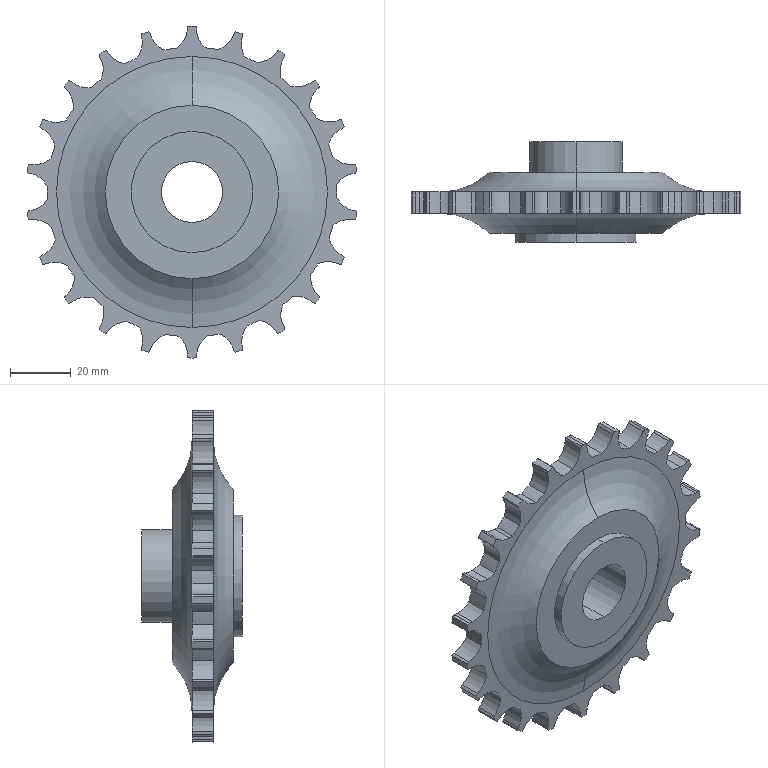Part | SolidWorks | features ICE 2, Extrusion 1, RefAxis 1, RevCut 1 | 1 solid | 159 faces | box 108.11 x 33 x 108.911 mm | volume 101426 mm3 | cylinder 149 | plane 6 | torus 4 | commonest cylinder face diameters 16 x50 3 x48 108.911 x23 95 x22 20 x2 30.405 x2